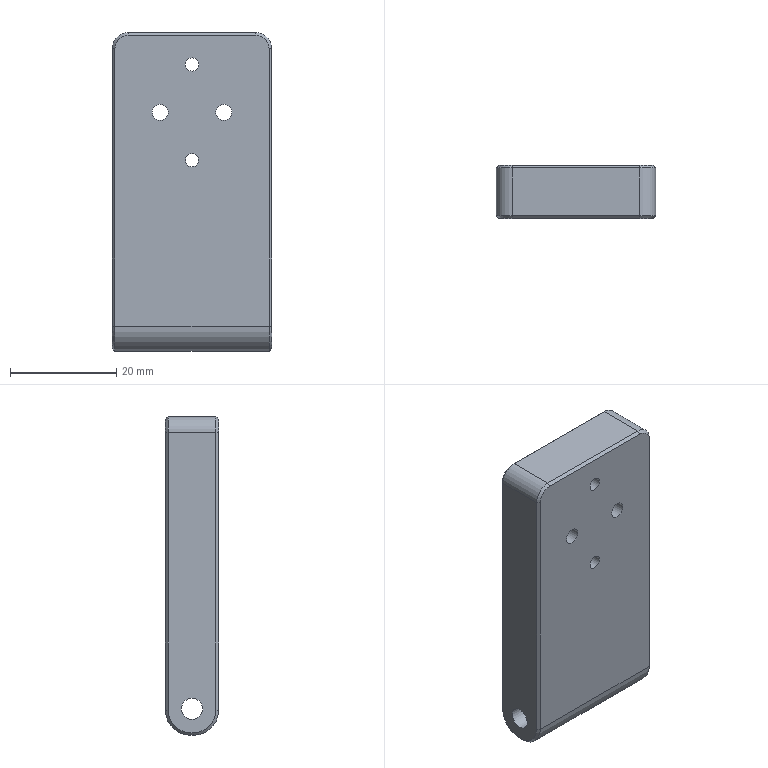CAM job | NX | 3+2 milling, drilling | part box 30 x 10 x 60 mm | stock box 35 x 12 x 65 mm
Tools:
number,name,description,diameter,corner_radius,flute_length,length,flutes
9,D10,平底铣刀-粗,10.0,0.0,35.0,75.0,2
7,D6-J,平底铣刀-精,6.0,0.0,25.0,75.0,2
19,D6R0.5,圆鼻刀-粗,6.0,0.5,50.0,75.0,2
1,D80R0.8飞刀,圆鼻刀-粗,80.0,0.8,50.0,75.0,2
1,D80R0.8飞刀-J,圆鼻刀-精,80.0,0.8,50.0,75.0,2
2,D6倒角刀,倒角刀,6.0,0.0,3.0,25.0,2
20,M3X0.5,丝锥,2.5,0.0,35.0,50.0,2
18,D3铰刀,Drilling Tool,3.0,0.0,75.0,100.0,6
12,钻头2.5,Twist Drill 2.5 mm,2.5,0.0,30.0,32.0,2
17,ZT2.9,Drilling Tool,2.9,0.0,35.0,50.0,2
Operations:
program,operation,operation_type,tool,method,geometry_group,spindle_rpm,surface_speed,feed_per_tooth,feed_cut,feed_plunge,cut_length_mm,path_length_mm,cut_time_min,machine_time_min
B,FLOORWALL_FACEMILL_ONECUT_ROUGH_COPY,VolumeBased25DMillingOperation,D80R0.8飞刀,LAYER_ROUGH-DEPTH_K-STEP_G,W-B,5000.0,1256.637,0.3,3000.0,100.0,1513.746,3025.967,0.5046,0.6558
B,FLOORWALL_FACEMILL_ONECUT_FINISH_COPY,VolumeBased25DMillingOperation,D80R0.8飞刀-J,SIDE_FINISH-DEPTH_K-STEP_G,W-B,5000.0,1256.637,0.1,1000.0,100.0,167.998,203.998,0.168,0.1716
B,ZLEVEL_FINISH_ZIGZAG_CLIMB_COPY_COPY,ZLevelMilling,D10,ZLEVEL_CLIMB-DEPTH_K-STEP_G,W-B,7000.0,131.947,0.3571,5000.0,100.0,3660.84,3689.296,0.7322,0.735
B,ZLEVEL_FINISH_ZIGZAG_CLIMB_COPY_COPY_COPY,ZLevelMilling,D6R0.5,ZLEVEL_CLIMB-DEPTH_K-STEP_G,W-B,7000.0,131.947,0.3571,5000.0,100.0,3370.147,3398.603,0.674,0.6769
B,DRILL_CHAMFER_3,Operation,D6倒角刀,METHOD,W-B,7000.0,131.947,0.0357,500.0,0.0,9.5,80.248,0.019,0.0261
B,DRILL_CHAMFER_4,Operation,D6倒角刀,METHOD,W-B,7000.0,131.947,0.0357,500.0,0.0,9.4,74.169,0.0188,0.0253
B,FLOORWALL_CHAMFER_COPY_1,VolumeBased25DMillingOperation,D6倒角刀,WALL_CLIMB_CHAMFER-DEPTH0-STEP_G,W-B,6500.0,122.519,0.1154,1500.0,100.0,150.933,190.333,0.1006,0.1046
A,TOPFACE,FaceMilling,D80R0.8飞刀,SIDE_FINISH-DEPTH_K-STEP_G,W-A,5000.0,1256.637,0.1,1000.0,100.0,154.0,190.0,0.154,0.1576
A,CAVITY_ROUGH-MED_COPY,CavityMilling,D10,LAYER_ROUGH-DEPTH_K-STEP_G,W-A,8000.0,251.32,0.25,4000.0,100.0,5892.886,6349.835,1.473,1.54
A,SPOT-DEPTH0.8,Operation,D6倒角刀,NONE,W-A,8000.0,150.796,0.0312,500.0,90.0,7.2,89.988,0.0144,0.0227
A,THRUHOLE-M3_TAPDRILL,Operation,钻头2.5,NONE,W-A,3000.0,23.562,0.05,300.0,90.0,33.502,126.032,0.1117,0.1209
A,THRUHOLE-PRECISION3.0_PREDRILL,Operation,ZT2.9,NONE,W-A,3200.0,29.154,0.0312,200.0,90.0,29.674,112.39,0.1484,0.1566
A,ZLEVEL_FINISH_ZIGZAG_CLIMB_COPY,ZLevelMilling,D6R0.5,ZLEVEL_CLIMB-DEPTH_K-STEP_G,W-A,7000.0,131.947,0.3571,5000.0,100.0,3519.83,3545.486,0.704,0.7065
A,DRILL_CHAMFER_1,Operation,D6倒角刀,METHOD,W-A,8000.0,150.796,0.0312,500.0,0.0,9.5,80.248,0.019,0.0261
A,DRILL_CHAMFER_2,Operation,D6倒角刀,METHOD,W-A,8000.0,150.796,0.0312,500.0,0.0,9.6,74.569,0.0192,0.0257
A,FLOORWALL_CHAMFER_COPY,VolumeBased25DMillingOperation,D6倒角刀,WALL_CLIMB_CHAMFER-DEPTH0-STEP_G,W-A,6500.0,122.519,0.1154,1500.0,100.0,156.664,196.064,0.1044,0.1084
A,THRUHOLE-TAP_M3,Operation,M3X0.5,METHOD,W-A,800.0,6.283,0.0003,0.5,90.0,28.0,115.028,56.0,56.009
A,REAM_HOLE,Operation,D3铰刀,METHOD,W-A,500.0,4.712,0.0167,50.0,0.0,24.0,101.042,0.48,0.4877
A,ZLEVEL_FINISH-MED_COPY,ZLevelMilling,D6-J,SIDE_FINISH-DEPTH_K-STEP_G,W-A,8000.0,150.792,0.0625,1000.0,100.0,401.714,430.433,0.4017,0.4046